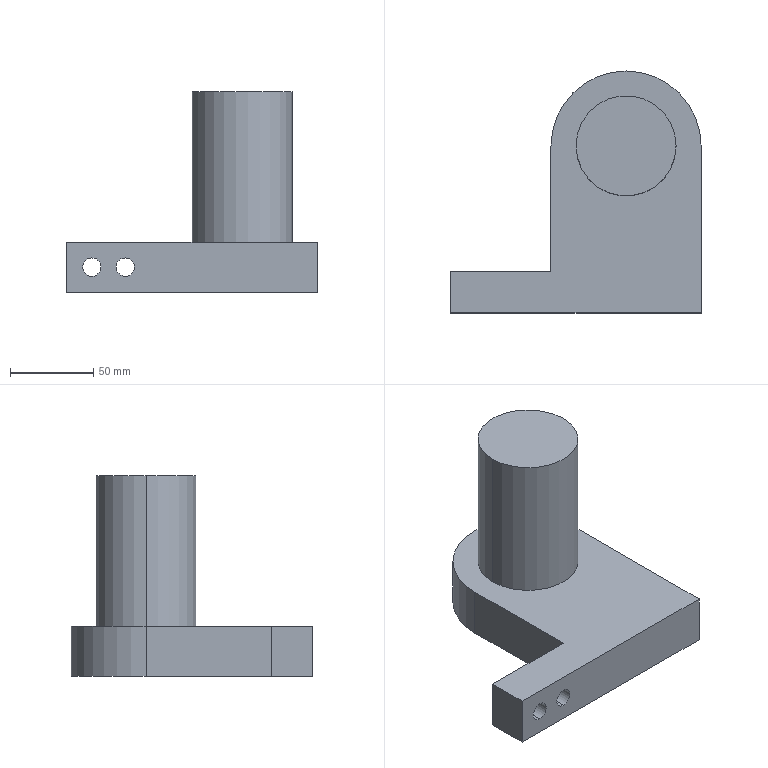Part | SolidWorks | features ICE 3, Extrusion 1 | 1 solid | 15 faces | box 150 x 145 x 120 mm | volume 660143 mm3 | plane 8 | cylinder 7 | commonest cylinder face diameters 11 x4 60 x2 90 x1
STEP:
#1=CARTESIAN_POINT('',(0.,87.5,105.));
#2=VERTEX_POINT('',#1);
#3=CARTESIAN_POINT('',(60.,87.5,105.));
#4=VERTEX_POINT('',#3);
#5=CARTESIAN_POINT('',(30.,87.5,105.));
#6=DIRECTION('',(0.,0.,-1.));
#7=DIRECTION('',(-1.,0.,0.));
#8=AXIS2_PLACEMENT_3D('',#5,#6,#7);
#9=CIRCLE('',#8,30.);
#10=EDGE_CURVE('',#2,#4,#9,.T.);
#11=ORIENTED_EDGE('',*,*,#10,.T.);
#12=CARTESIAN_POINT('',(60.,87.5,15.));
#13=VERTEX_POINT('',#12);
#14=CARTESIAN_POINT('',(60.,87.5,105.));
#15=DIRECTION('',(0.,0.,-1.));
#16=VECTOR('',#15,1000.);
#17=LINE('',#14,#16);
#18=EDGE_CURVE('',#4,#13,#17,.T.);
#19=ORIENTED_EDGE('',*,*,#18,.T.);
#20=CARTESIAN_POINT('',(0.,87.5,15.));
#21=VERTEX_POINT('',#20);
#22=CARTESIAN_POINT('',(30.,87.5,15.));
#23=DIRECTION('',(0.,0.,1.));
#24=DIRECTION('',(1.,0.,0.));
#25=AXIS2_PLACEMENT_3D('',#22,#23,#24);
#26=CIRCLE('',#25,30.);
#27=EDGE_CURVE('',#13,#21,#26,.T.);
#28=ORIENTED_EDGE('',*,*,#27,.T.);
#29=CARTESIAN_POINT('',(0.,87.5,105.));
#30=DIRECTION('',(0.,0.,-1.));
#31=VECTOR('',#30,1000.);
#32=LINE('',#29,#31);
#33=EDGE_CURVE('',#2,#21,#32,.T.);
#34=ORIENTED_EDGE('',*,*,#33,.F.);
#35=EDGE_LOOP('',(#11,#19,#28,#34));
#36=FACE_OUTER_BOUND('',#35,.T.);
#37=CARTESIAN_POINT('',(30.,87.5,105.));
#38=DIRECTION('',(0.,0.,-1.));
#39=DIRECTION('',(-1.,0.,0.));
#40=AXIS2_PLACEMENT_3D('',#37,#38,#39);
#41=CYLINDRICAL_SURFACE('',#40,30.);
#42=ADVANCED_FACE('',(#36),#41,.T.);
#43=CARTESIAN_POINT('',(-60.,-12.5,-5.5));
#44=VERTEX_POINT('',#43);
#45=CARTESIAN_POINT('',(-60.,-12.5,5.5));
#46=VERTEX_POINT('',#45);
#47=CARTESIAN_POINT('',(-60.,-12.5,0.));
#48=DIRECTION('',(0.,1.,0.));
#49=DIRECTION('',(0.,0.,1.));
#50=AXIS2_PLACEMENT_3D('',#47,#48,#49);
#51=CIRCLE('',#50,5.5);
#52=EDGE_CURVE('',#44,#46,#51,.T.);
#53=ORIENTED_EDGE('',*,*,#52,.F.);
#54=CARTESIAN_POINT('',(-60.,12.5,-5.5));
#55=VERTEX_POINT('',#54);
#56=CARTESIAN_POINT('',(-60.,-17.5,-5.5));
#57=DIRECTION('',(0.,1.,0.));
#58=VECTOR('',#57,1000.);
#59=LINE('',#56,#58);
#60=EDGE_CURVE('',#44,#55,#59,.T.);
#61=ORIENTED_EDGE('',*,*,#60,.T.);
#62=CARTESIAN_POINT('',(-60.,12.5,5.5));
#63=VERTEX_POINT('',#62);
#64=CARTESIAN_POINT('',(-60.,12.5,0.));
#65=DIRECTION('',(0.,1.,0.));
#66=DIRECTION('',(0.,0.,1.));
#67=AXIS2_PLACEMENT_3D('',#64,#65,#66);
#68=CIRCLE('',#67,5.5);
#69=EDGE_CURVE('',#55,#63,#68,.T.);
#70=ORIENTED_EDGE('',*,*,#69,.T.);
#71=CARTESIAN_POINT('',(-60.,-17.5,5.5));
#72=DIRECTION('',(0.,1.,0.));
#73=VECTOR('',#72,1000.);
#74=LINE('',#71,#73);
#75=EDGE_CURVE('',#46,#63,#74,.T.);
#76=ORIENTED_EDGE('',*,*,#75,.F.);
#77=EDGE_LOOP('',(#53,#61,#70,#76));
#78=FACE_OUTER_BOUND('',#77,.T.);
#79=CARTESIAN_POINT('',(-60.,-17.5,0.));
#80=DIRECTION('',(0.,1.,0.));
#81=DIRECTION('',(0.,0.,1.));
#82=AXIS2_PLACEMENT_3D('',#79,#80,#81);
#83=CYLINDRICAL_SURFACE('',#82,5.5);
#84=ADVANCED_FACE('',(#78),#83,.F.);
#85=CARTESIAN_POINT('',(-40.,-12.5,-5.5));
#86=VERTEX_POINT('',#85);
#87=CARTESIAN_POINT('',(-40.,-12.5,5.5));
#88=VERTEX_POINT('',#87);
#89=CARTESIAN_POINT('',(-40.,-12.5,0.));
#90=DIRECTION('',(0.,1.,0.));
#91=DIRECTION('',(0.,0.,1.));
#92=AXIS2_PLACEMENT_3D('',#89,#90,#91);
#93=CIRCLE('',#92,5.5);
#94=EDGE_CURVE('',#86,#88,#93,.T.);
#95=ORIENTED_EDGE('',*,*,#94,.F.);
#96=CARTESIAN_POINT('',(-40.,12.5,-5.5));
#97=VERTEX_POINT('',#96);
#98=CARTESIAN_POINT('',(-40.,-17.5,-5.5));
#99=DIRECTION('',(0.,1.,0.));
#100=VECTOR('',#99,1000.);
#101=LINE('',#98,#100);
#102=EDGE_CURVE('',#86,#97,#101,.T.);
#103=ORIENTED_EDGE('',*,*,#102,.T.);
#104=CARTESIAN_POINT('',(-40.,12.5,5.5));
#105=VERTEX_POINT('',#104);
#106=CARTESIAN_POINT('',(-40.,12.5,0.));
#107=DIRECTION('',(0.,1.,0.));
#108=DIRECTION('',(0.,0.,1.));
#109=AXIS2_PLACEMENT_3D('',#106,#107,#108);
#110=CIRCLE('',#109,5.5);
#111=EDGE_CURVE('',#97,#105,#110,.T.);
#112=ORIENTED_EDGE('',*,*,#111,.T.);
#113=CARTESIAN_POINT('',(-40.,-17.5,5.5));
#114=DIRECTION('',(0.,1.,0.));
#115=VECTOR('',#114,1000.);
#116=LINE('',#113,#115);
#117=EDGE_CURVE('',#88,#105,#116,.T.);
#118=ORIENTED_EDGE('',*,*,#117,.F.);
#119=EDGE_LOOP('',(#95,#103,#112,#118));
#120=FACE_OUTER_BOUND('',#119,.T.);
#121=CARTESIAN_POINT('',(-40.,-17.5,0.));
#122=DIRECTION('',(0.,1.,0.));
#123=DIRECTION('',(0.,0.,1.));
#124=AXIS2_PLACEMENT_3D('',#121,#122,#123);
#125=CYLINDRICAL_SURFACE('',#124,5.5);
#126=ADVANCED_FACE('',(#120),#125,.F.);
#127=CARTESIAN_POINT('',(75.,-12.5,-15.));
#128=VERTEX_POINT('',#127);
#129=CARTESIAN_POINT('',(75.,87.5,-15.));
#130=VERTEX_POINT('',#129);
#131=CARTESIAN_POINT('',(75.,12.5,-15.));
#132=DIRECTION('',(0.,1.,0.));
#133=VECTOR('',#132,1000.);
#134=LINE('',#131,#133);
#135=EDGE_CURVE('',#128,#130,#134,.T.);
#136=ORIENTED_EDGE('',*,*,#135,.T.);
#137=CARTESIAN_POINT('',(75.,87.5,15.));
#138=VERTEX_POINT('',#137);
#139=CARTESIAN_POINT('',(75.,87.5,-175.176));
#140=DIRECTION('',(0.,0.,1.));
#141=VECTOR('',#140,1000.);
#142=LINE('',#139,#141);
#143=EDGE_CURVE('',#130,#138,#142,.T.);
#144=ORIENTED_EDGE('',*,*,#143,.T.);
#145=CARTESIAN_POINT('',(75.,-12.5,15.));
#146=VERTEX_POINT('',#145);
#147=CARTESIAN_POINT('',(75.,12.5,15.));
#148=DIRECTION('',(0.,1.,0.));
#149=VECTOR('',#148,1000.);
#150=LINE('',#147,#149);
#151=EDGE_CURVE('',#146,#138,#150,.T.);
#152=ORIENTED_EDGE('',*,*,#151,.F.);
#153=CARTESIAN_POINT('',(75.,-12.5,15.));
#154=DIRECTION('',(0.,0.,-1.));
#155=VECTOR('',#154,1000.);
#156=LINE('',#153,#155);
#157=EDGE_CURVE('',#146,#128,#156,.T.);
#158=ORIENTED_EDGE('',*,*,#157,.T.);
#159=EDGE_LOOP('',(#136,#144,#152,#158));
#160=FACE_OUTER_BOUND('',#159,.T.);
#161=CARTESIAN_POINT('',(75.,12.5,15.));
#162=DIRECTION('',(-1.,0.,0.));
#163=DIRECTION('',(0.,0.,1.));
#164=AXIS2_PLACEMENT_3D('',#161,#162,#163);
#165=PLANE('',#164);
#166=ADVANCED_FACE('',(#160),#165,.F.);
#167=CARTESIAN_POINT('',(-60.,12.5,0.));
#168=DIRECTION('',(0.,1.,0.));
#169=DIRECTION('',(0.,0.,1.));
#170=AXIS2_PLACEMENT_3D('',#167,#168,#169);
#171=CIRCLE('',#170,5.5);
#172=EDGE_CURVE('',#63,#55,#171,.T.);
#173=ORIENTED_EDGE('',*,*,#172,.F.);
#174=ORIENTED_EDGE('',*,*,#69,.F.);
#175=EDGE_LOOP('',(#173,#174));
#176=FACE_BOUND('',#175,.T.);
#177=CARTESIAN_POINT('',(-40.,12.5,0.));
#178=DIRECTION('',(0.,1.,0.));
#179=DIRECTION('',(0.,0.,1.));
#180=AXIS2_PLACEMENT_3D('',#177,#178,#179);
#181=CIRCLE('',#180,5.5);
#182=EDGE_CURVE('',#105,#97,#181,.T.);
#183=ORIENTED_EDGE('',*,*,#182,.F.);
#184=ORIENTED_EDGE('',*,*,#111,.F.);
#185=EDGE_LOOP('',(#183,#184));
#186=FACE_BOUND('',#185,.T.);
#187=CARTESIAN_POINT('',(-15.,12.5,15.));
#188=VERTEX_POINT('',#187);
#189=CARTESIAN_POINT('',(-75.,12.5,15.));
#190=VERTEX_POINT('',#189);
#191=CARTESIAN_POINT('',(-75.,12.5,15.));
#192=DIRECTION('',(-1.,0.,0.));
#193=VECTOR('',#192,1000.);
#194=LINE('',#191,#193);
#195=EDGE_CURVE('',#188,#190,#194,.T.);
#196=ORIENTED_EDGE('',*,*,#195,.F.);
#197=CARTESIAN_POINT('',(-15.,12.5,-15.));
#198=VERTEX_POINT('',#197);
#199=CARTESIAN_POINT('',(-15.,12.5,15.));
#200=DIRECTION('',(0.,0.,-1.));
#201=VECTOR('',#200,1000.);
#202=LINE('',#199,#201);
#203=EDGE_CURVE('',#188,#198,#202,.T.);
#204=ORIENTED_EDGE('',*,*,#203,.T.);
#205=CARTESIAN_POINT('',(-75.,12.5,-15.));
#206=VERTEX_POINT('',#205);
#207=CARTESIAN_POINT('',(-75.,12.5,-15.));
#208=DIRECTION('',(-1.,0.,0.));
#209=VECTOR('',#208,1000.);
#210=LINE('',#207,#209);
#211=EDGE_CURVE('',#198,#206,#210,.T.);
#212=ORIENTED_EDGE('',*,*,#211,.T.);
#213=CARTESIAN_POINT('',(-75.,12.5,15.));
#214=DIRECTION('',(0.,0.,-1.));
#215=VECTOR('',#214,1000.);
#216=LINE('',#213,#215);
#217=EDGE_CURVE('',#190,#206,#216,.T.);
#218=ORIENTED_EDGE('',*,*,#217,.F.);
#219=EDGE_LOOP('',(#196,#204,#212,#218));
#220=FACE_OUTER_BOUND('',#219,.T.);
#221=CARTESIAN_POINT('',(-75.,12.5,15.));
#222=DIRECTION('',(0.,-1.,0.));
#223=DIRECTION('',(0.,0.,-1.));
#224=AXIS2_PLACEMENT_3D('',#221,#222,#223);
#225=PLANE('',#224);
#226=ADVANCED_FACE('',(#176,#186,#220),#225,.F.);
#227=CARTESIAN_POINT('',(-75.,-12.5,-15.));
#228=VERTEX_POINT('',#227);
#229=CARTESIAN_POINT('',(-75.,12.5,-15.));
#230=DIRECTION('',(0.,-1.,0.));
#231=VECTOR('',#230,1000.);
#232=LINE('',#229,#231);
#233=EDGE_CURVE('',#206,#228,#232,.T.);
#234=ORIENTED_EDGE('',*,*,#233,.T.);
#235=CARTESIAN_POINT('',(-75.,-12.5,15.));
#236=VERTEX_POINT('',#235);
#237=CARTESIAN_POINT('',(-75.,-12.5,15.));
#238=DIRECTION('',(0.,0.,-1.));
#239=VECTOR('',#238,1000.);
#240=LINE('',#237,#239);
#241=EDGE_CURVE('',#236,#228,#240,.T.);
#242=ORIENTED_EDGE('',*,*,#241,.F.);
#243=CARTESIAN_POINT('',(-75.,12.5,15.));
#244=DIRECTION('',(0.,-1.,0.));
#245=VECTOR('',#244,1000.);
#246=LINE('',#243,#245);
#247=EDGE_CURVE('',#190,#236,#246,.T.);
#248=ORIENTED_EDGE('',*,*,#247,.F.);
#249=ORIENTED_EDGE('',*,*,#217,.T.);
#250=EDGE_LOOP('',(#234,#242,#248,#249));
#251=FACE_OUTER_BOUND('',#250,.T.);
#252=CARTESIAN_POINT('',(-75.,12.5,15.));
#253=DIRECTION('',(1.,0.,0.));
#254=DIRECTION('',(0.,0.,-1.));
#255=AXIS2_PLACEMENT_3D('',#252,#253,#254);
#256=PLANE('',#255);
#257=ADVANCED_FACE('',(#251),#256,.F.);
#258=CARTESIAN_POINT('',(-60.,-12.5,0.));
#259=DIRECTION('',(0.,1.,0.));
#260=DIRECTION('',(0.,0.,1.));
#261=AXIS2_PLACEMENT_3D('',#258,#259,#260);
#262=CIRCLE('',#261,5.5);
#263=EDGE_CURVE('',#46,#44,#262,.T.);
#264=ORIENTED_EDGE('',*,*,#263,.T.);
#265=ORIENTED_EDGE('',*,*,#52,.T.);
#266=EDGE_LOOP('',(#264,#265));
#267=FACE_BOUND('',#266,.T.);
#268=CARTESIAN_POINT('',(-40.,-12.5,0.));
#269=DIRECTION('',(0.,1.,0.));
#270=DIRECTION('',(0.,0.,1.));
#271=AXIS2_PLACEMENT_3D('',#268,#269,#270);
#272=CIRCLE('',#271,5.5);
#273=EDGE_CURVE('',#88,#86,#272,.T.);
#274=ORIENTED_EDGE('',*,*,#273,.T.);
#275=ORIENTED_EDGE('',*,*,#94,.T.);
#276=EDGE_LOOP('',(#274,#275));
#277=FACE_BOUND('',#276,.T.);
#278=CARTESIAN_POINT('',(-75.,-12.5,-15.));
#279=DIRECTION('',(1.,0.,0.));
#280=VECTOR('',#279,1000.);
#281=LINE('',#278,#280);
#282=EDGE_CURVE('',#228,#128,#281,.T.);
#283=ORIENTED_EDGE('',*,*,#282,.T.);
#284=ORIENTED_EDGE('',*,*,#157,.F.);
#285=CARTESIAN_POINT('',(-75.,-12.5,15.));
#286=DIRECTION('',(1.,0.,0.));
#287=VECTOR('',#286,1000.);
#288=LINE('',#285,#287);
#289=EDGE_CURVE('',#236,#146,#288,.T.);
#290=ORIENTED_EDGE('',*,*,#289,.F.);
#291=ORIENTED_EDGE('',*,*,#241,.T.);
#292=EDGE_LOOP('',(#283,#284,#290,#291));
#293=FACE_OUTER_BOUND('',#292,.T.);
#294=CARTESIAN_POINT('',(-75.,-12.5,15.));
#295=DIRECTION('',(0.,1.,0.));
#296=DIRECTION('',(0.,0.,1.));
#297=AXIS2_PLACEMENT_3D('',#294,#295,#296);
#298=PLANE('',#297);
#299=ADVANCED_FACE('',(#267,#277,#293),#298,.F.);
#300=ORIENTED_EDGE('',*,*,#151,.T.);
#301=CARTESIAN_POINT('',(-15.,87.5,15.));
#302=VERTEX_POINT('',#301);
#303=CARTESIAN_POINT('',(30.,87.5,15.));
#304=DIRECTION('',(0.,0.,1.));
#305=DIRECTION('',(1.,0.,0.));
#306=AXIS2_PLACEMENT_3D('',#303,#304,#305);
#307=CIRCLE('',#306,45.);
#308=EDGE_CURVE('',#138,#302,#307,.T.);
#309=ORIENTED_EDGE('',*,*,#308,.T.);
#310=CARTESIAN_POINT('',(-15.,87.5,15.));
#311=DIRECTION('',(0.,-1.,0.));
#312=VECTOR('',#311,1000.);
#313=LINE('',#310,#312);
#314=EDGE_CURVE('',#302,#188,#313,.T.);
#315=ORIENTED_EDGE('',*,*,#314,.T.);
#316=ORIENTED_EDGE('',*,*,#195,.T.);
#317=ORIENTED_EDGE('',*,*,#247,.T.);
#318=ORIENTED_EDGE('',*,*,#289,.T.);
#319=EDGE_LOOP('',(#300,#309,#315,#316,#317,#318));
#320=FACE_OUTER_BOUND('',#319,.T.);
#321=CARTESIAN_POINT('',(30.,87.5,15.));
#322=DIRECTION('',(0.,0.,1.));
#323=DIRECTION('',(1.,0.,0.));
#324=AXIS2_PLACEMENT_3D('',#321,#322,#323);
#325=CIRCLE('',#324,30.);
#326=EDGE_CURVE('',#21,#13,#325,.T.);
#327=ORIENTED_EDGE('',*,*,#326,.F.);
#328=ORIENTED_EDGE('',*,*,#27,.F.);
#329=EDGE_LOOP('',(#327,#328));
#330=FACE_BOUND('',#329,.T.);
#331=CARTESIAN_POINT('',(0.,0.,15.));
#332=DIRECTION('',(0.,0.,1.));
#333=DIRECTION('',(1.,0.,0.));
#334=AXIS2_PLACEMENT_3D('',#331,#332,#333);
#335=PLANE('',#334);
#336=ADVANCED_FACE('',(#320,#330),#335,.T.);
#337=ORIENTED_EDGE('',*,*,#211,.F.);
#338=CARTESIAN_POINT('',(-15.,87.5,-15.));
#339=VERTEX_POINT('',#338);
#340=CARTESIAN_POINT('',(-15.,87.5,-15.));
#341=DIRECTION('',(0.,1.,0.));
#342=VECTOR('',#341,1000.);
#343=LINE('',#340,#342);
#344=EDGE_CURVE('',#198,#339,#343,.T.);
#345=ORIENTED_EDGE('',*,*,#344,.T.);
#346=CARTESIAN_POINT('',(30.,87.5,-15.));
#347=DIRECTION('',(0.,0.,-1.));
#348=DIRECTION('',(1.,0.,0.));
#349=AXIS2_PLACEMENT_3D('',#346,#347,#348);
#350=CIRCLE('',#349,45.);
#351=EDGE_CURVE('',#339,#130,#350,.T.);
#352=ORIENTED_EDGE('',*,*,#351,.T.);
#353=ORIENTED_EDGE('',*,*,#135,.F.);
#354=ORIENTED_EDGE('',*,*,#282,.F.);
#355=ORIENTED_EDGE('',*,*,#233,.F.);
#356=EDGE_LOOP('',(#337,#345,#352,#353,#354,#355));
#357=FACE_OUTER_BOUND('',#356,.T.);
#358=CARTESIAN_POINT('',(0.,0.,-15.));
#359=DIRECTION('',(0.,0.,1.));
#360=DIRECTION('',(1.,0.,0.));
#361=AXIS2_PLACEMENT_3D('',#358,#359,#360);
#362=PLANE('',#361);
#363=ADVANCED_FACE('',(#357),#362,.F.);
#364=ORIENTED_EDGE('',*,*,#203,.F.);
#365=ORIENTED_EDGE('',*,*,#314,.F.);
#366=CARTESIAN_POINT('',(-15.,87.5,-175.176));
#367=DIRECTION('',(0.,0.,1.));
#368=VECTOR('',#367,1000.);
#369=LINE('',#366,#368);
#370=EDGE_CURVE('',#339,#302,#369,.T.);
#371=ORIENTED_EDGE('',*,*,#370,.F.);
#372=ORIENTED_EDGE('',*,*,#344,.F.);
#373=EDGE_LOOP('',(#364,#365,#371,#372));
#374=FACE_OUTER_BOUND('',#373,.T.);
#375=CARTESIAN_POINT('',(-15.,87.5,-175.176));
#376=DIRECTION('',(-1.,0.,0.));
#377=DIRECTION('',(0.,0.,1.));
#378=AXIS2_PLACEMENT_3D('',#375,#376,#377);
#379=PLANE('',#378);
#380=ADVANCED_FACE('',(#374),#379,.T.);
#381=ORIENTED_EDGE('',*,*,#351,.F.);
#382=ORIENTED_EDGE('',*,*,#370,.T.);
#383=ORIENTED_EDGE('',*,*,#308,.F.);
#384=ORIENTED_EDGE('',*,*,#143,.F.);
#385=EDGE_LOOP('',(#381,#382,#383,#384));
#386=FACE_OUTER_BOUND('',#385,.T.);
#387=CARTESIAN_POINT('',(30.,87.5,-175.176));
#388=DIRECTION('',(0.,0.,1.));
#389=DIRECTION('',(1.,0.,0.));
#390=AXIS2_PLACEMENT_3D('',#387,#388,#389);
#391=CYLINDRICAL_SURFACE('',#390,45.);
#392=ADVANCED_FACE('',(#386),#391,.T.);
#393=ORIENTED_EDGE('',*,*,#102,.F.);
#394=ORIENTED_EDGE('',*,*,#273,.F.);
#395=ORIENTED_EDGE('',*,*,#117,.T.);
#396=ORIENTED_EDGE('',*,*,#182,.T.);
#397=EDGE_LOOP('',(#393,#394,#395,#396));
#398=FACE_OUTER_BOUND('',#397,.T.);
#399=CARTESIAN_POINT('',(-40.,-17.5,0.));
#400=DIRECTION('',(0.,1.,0.));
#401=DIRECTION('',(0.,0.,1.));
#402=AXIS2_PLACEMENT_3D('',#399,#400,#401);
#403=CYLINDRICAL_SURFACE('',#402,5.5);
#404=ADVANCED_FACE('',(#398),#403,.F.);
#405=ORIENTED_EDGE('',*,*,#60,.F.);
#406=ORIENTED_EDGE('',*,*,#263,.F.);
#407=ORIENTED_EDGE('',*,*,#75,.T.);
#408=ORIENTED_EDGE('',*,*,#172,.T.);
#409=EDGE_LOOP('',(#405,#406,#407,#408));
#410=FACE_OUTER_BOUND('',#409,.T.);
#411=CARTESIAN_POINT('',(-60.,-17.5,0.));
#412=DIRECTION('',(0.,1.,0.));
#413=DIRECTION('',(0.,0.,1.));
#414=AXIS2_PLACEMENT_3D('',#411,#412,#413);
#415=CYLINDRICAL_SURFACE('',#414,5.5);
#416=ADVANCED_FACE('',(#410),#415,.F.);
#417=ORIENTED_EDGE('',*,*,#18,.F.);
#418=CARTESIAN_POINT('',(30.,87.5,105.));
#419=DIRECTION('',(0.,0.,-1.));
#420=DIRECTION('',(-1.,0.,0.));
#421=AXIS2_PLACEMENT_3D('',#418,#419,#420);
#422=CIRCLE('',#421,30.);
#423=EDGE_CURVE('',#4,#2,#422,.T.);
#424=ORIENTED_EDGE('',*,*,#423,.T.);
#425=ORIENTED_EDGE('',*,*,#33,.T.);
#426=ORIENTED_EDGE('',*,*,#326,.T.);
#427=EDGE_LOOP('',(#417,#424,#425,#426));
#428=FACE_OUTER_BOUND('',#427,.T.);
#429=CARTESIAN_POINT('',(30.,87.5,105.));
#430=DIRECTION('',(0.,0.,-1.));
#431=DIRECTION('',(-1.,0.,0.));
#432=AXIS2_PLACEMENT_3D('',#429,#430,#431);
#433=CYLINDRICAL_SURFACE('',#432,30.);
#434=ADVANCED_FACE('',(#428),#433,.T.);
#435=ORIENTED_EDGE('',*,*,#10,.F.);
#436=ORIENTED_EDGE('',*,*,#423,.F.);
#437=EDGE_LOOP('',(#435,#436));
#438=FACE_OUTER_BOUND('',#437,.T.);
#439=CARTESIAN_POINT('',(30.,87.5,105.));
#440=DIRECTION('',(0.,0.,-1.));
#441=DIRECTION('',(-1.,0.,0.));
#442=AXIS2_PLACEMENT_3D('',#439,#440,#441);
#443=PLANE('',#442);
#444=ADVANCED_FACE('',(#438),#443,.F.);
#445=CLOSED_SHELL('',(#42,#84,#126,#166,#226,#257,#299,#336,#363,#380,#392,#404,#416,#434,#444));
#446=MANIFOLD_SOLID_BREP('',#445);
#447=CARTESIAN_POINT('',(0.,0.,0.));
#448=DIRECTION('',(0.,0.,1.));
#449=DIRECTION('',(1.,0.,0.));
#450=AXIS2_PLACEMENT_3D('',#447,#448,#449);
#451=(LENGTH_UNIT()NAMED_UNIT(*)SI_UNIT(.MILLI.,.METRE.));
#452=UNCERTAINTY_MEASURE_WITH_UNIT(LENGTH_MEASURE(0.00001),#451,'','');
#453=(NAMED_UNIT(*)PLANE_ANGLE_UNIT()SI_UNIT($,.RADIAN.));
#454=(NAMED_UNIT(*)SI_UNIT($,.STERADIAN.)SOLID_ANGLE_UNIT());
#455=(GEOMETRIC_REPRESENTATION_CONTEXT(3)GLOBAL_UNCERTAINTY_ASSIGNED_CONTEXT((#452))GLOBAL_UNIT_ASSIGNED_CONTEXT((#451,#453,#454))REPRESENTATION_CONTEXT('',''));
#456=ADVANCED_BREP_SHAPE_REPRESENTATION('',(#446,#450),#455);